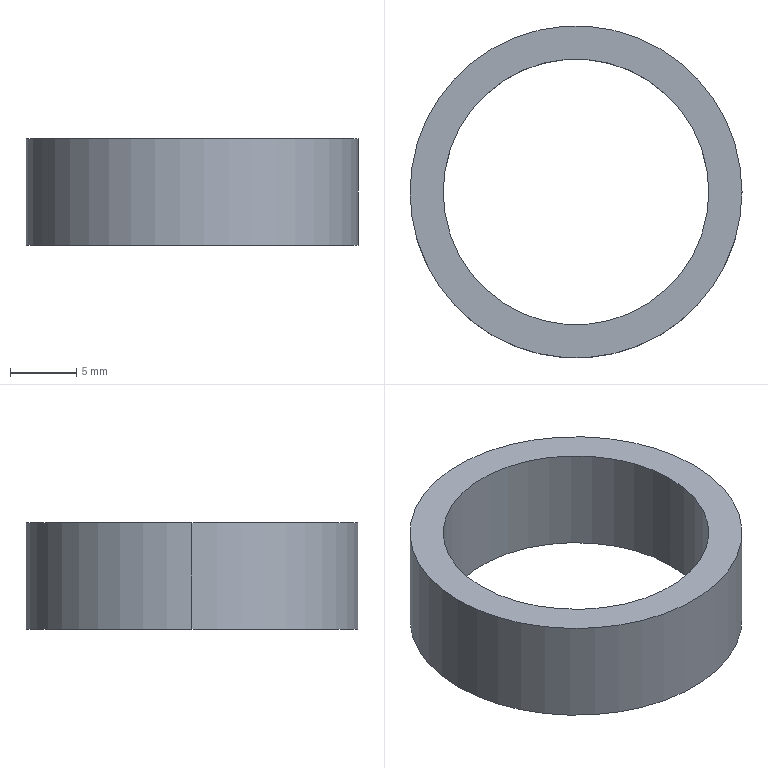Part | STEP file | BCC3 H16_5 | 1 solid | 6 faces | box 25 x 25 x 8 mm | volume 1414 mm3 | cylinder 4 | plane 2 | commonest cylinder face diameters 20 x2 25 x2
STEP:
#1=CARTESIAN_POINT('',(0.,0.,0.));
#2=DIRECTION('',(0.,0.,1.));
#3=DIRECTION('',(1.,0.,0.));
#4=AXIS2_PLACEMENT_3D('',#1,#2,#3);
#5=CARTESIAN_POINT('',(-10.,0.,8.));
#6=VERTEX_POINT('',#5);
#7=CARTESIAN_POINT('',(-10.,0.,0.));
#8=VERTEX_POINT('',#7);
#9=CARTESIAN_POINT('',(-10.,0.,8.));
#10=DIRECTION('',(0.,0.,-1.));
#11=VECTOR('',#10,1.);
#12=LINE('',#9,#11);
#13=CARTESIAN_POINT('',(0.,0.,8.));
#14=DIRECTION('',(0.,0.,-1.));
#15=DIRECTION('',(-1.,0.,0.));
#16=AXIS2_PLACEMENT_3D('',#13,#14,#15);
#17=CYLINDRICAL_SURFACE('',#16,10.);
#18=CARTESIAN_POINT('',(6.283,0.));
#19=DIRECTION('',(0.,1.));
#20=VECTOR('',#19,1.);
#21=LINE('',#18,#20);
#22=(GEOMETRIC_REPRESENTATION_CONTEXT(2)PARAMETRIC_REPRESENTATION_CONTEXT()REPRESENTATION_CONTEXT('',''));
#23=DEFINITIONAL_REPRESENTATION('',(#21),#22);
#24=PCURVE('',#17,#23);
#25=CARTESIAN_POINT('',(0.,0.,8.));
#26=DIRECTION('',(0.,0.,-1.));
#27=DIRECTION('',(-1.,0.,0.));
#28=AXIS2_PLACEMENT_3D('',#25,#26,#27);
#29=CYLINDRICAL_SURFACE('',#28,10.);
#30=CARTESIAN_POINT('',(0.,0.));
#31=DIRECTION('',(0.,1.));
#32=VECTOR('',#31,1.);
#33=LINE('',#30,#32);
#34=(GEOMETRIC_REPRESENTATION_CONTEXT(2)PARAMETRIC_REPRESENTATION_CONTEXT()REPRESENTATION_CONTEXT('',''));
#35=DEFINITIONAL_REPRESENTATION('',(#33),#34);
#36=PCURVE('',#29,#35);
#37=SURFACE_CURVE('',#12,(#24,#36),.PCURVE_S1.);
#38=EDGE_CURVE('',#6,#8,#37,.T.);
#39=ORIENTED_EDGE('',*,*,#38,.T.);
#40=CARTESIAN_POINT('',(10.,0.,0.));
#41=VERTEX_POINT('',#40);
#42=CARTESIAN_POINT('',(0.,0.,0.));
#43=DIRECTION('',(0.,0.,1.));
#44=DIRECTION('',(1.,0.,0.));
#45=AXIS2_PLACEMENT_3D('',#42,#43,#44);
#46=CIRCLE('',#45,10.);
#47=CARTESIAN_POINT('',(9.425,8.));
#48=DIRECTION('',(-1.,0.));
#49=VECTOR('',#48,1.);
#50=LINE('',#47,#49);
#51=(GEOMETRIC_REPRESENTATION_CONTEXT(2)PARAMETRIC_REPRESENTATION_CONTEXT()REPRESENTATION_CONTEXT('',''));
#52=DEFINITIONAL_REPRESENTATION('',(#50),#51);
#53=PCURVE('',#17,#52);
#54=CARTESIAN_POINT('',(0.,0.,0.));
#55=DIRECTION('',(0.,0.,1.));
#56=DIRECTION('',(1.,0.,0.));
#57=AXIS2_PLACEMENT_3D('',#54,#55,#56);
#58=PLANE('',#57);
#59=CARTESIAN_POINT('',(0.,0.));
#60=DIRECTION('',(1.,0.));
#61=AXIS2_PLACEMENT_2D('',#59,#60);
#62=CIRCLE('',#61,10.);
#63=(GEOMETRIC_REPRESENTATION_CONTEXT(2)PARAMETRIC_REPRESENTATION_CONTEXT()REPRESENTATION_CONTEXT('',''));
#64=DEFINITIONAL_REPRESENTATION('',(#62),#63);
#65=PCURVE('',#58,#64);
#66=SURFACE_CURVE('',#46,(#53,#65),.PCURVE_S1.);
#67=EDGE_CURVE('',#8,#41,#66,.T.);
#68=ORIENTED_EDGE('',*,*,#67,.T.);
#69=CARTESIAN_POINT('',(10.,0.,8.));
#70=VERTEX_POINT('',#69);
#71=CARTESIAN_POINT('',(10.,0.,8.));
#72=DIRECTION('',(0.,0.,-1.));
#73=VECTOR('',#72,1.);
#74=LINE('',#71,#73);
#75=CARTESIAN_POINT('',(3.142,0.));
#76=DIRECTION('',(0.,1.));
#77=VECTOR('',#76,1.);
#78=LINE('',#75,#77);
#79=(GEOMETRIC_REPRESENTATION_CONTEXT(2)PARAMETRIC_REPRESENTATION_CONTEXT()REPRESENTATION_CONTEXT('',''));
#80=DEFINITIONAL_REPRESENTATION('',(#78),#79);
#81=PCURVE('',#17,#80);
#82=CARTESIAN_POINT('',(3.142,0.));
#83=DIRECTION('',(0.,1.));
#84=VECTOR('',#83,1.);
#85=LINE('',#82,#84);
#86=(GEOMETRIC_REPRESENTATION_CONTEXT(2)PARAMETRIC_REPRESENTATION_CONTEXT()REPRESENTATION_CONTEXT('',''));
#87=DEFINITIONAL_REPRESENTATION('',(#85),#86);
#88=PCURVE('',#29,#87);
#89=SURFACE_CURVE('',#74,(#81,#88),.PCURVE_S1.);
#90=EDGE_CURVE('',#70,#41,#89,.T.);
#91=ORIENTED_EDGE('',*,*,#90,.F.);
#92=CARTESIAN_POINT('',(0.,0.,8.));
#93=DIRECTION('',(0.,0.,1.));
#94=DIRECTION('',(1.,0.,0.));
#95=AXIS2_PLACEMENT_3D('',#92,#93,#94);
#96=CIRCLE('',#95,10.);
#97=CARTESIAN_POINT('',(9.425,0.));
#98=DIRECTION('',(-1.,0.));
#99=VECTOR('',#98,1.);
#100=LINE('',#97,#99);
#101=(GEOMETRIC_REPRESENTATION_CONTEXT(2)PARAMETRIC_REPRESENTATION_CONTEXT()REPRESENTATION_CONTEXT('',''));
#102=DEFINITIONAL_REPRESENTATION('',(#100),#101);
#103=PCURVE('',#17,#102);
#104=CARTESIAN_POINT('',(0.,0.,8.));
#105=DIRECTION('',(0.,0.,1.));
#106=DIRECTION('',(1.,0.,0.));
#107=AXIS2_PLACEMENT_3D('',#104,#105,#106);
#108=PLANE('',#107);
#109=CARTESIAN_POINT('',(0.,0.));
#110=DIRECTION('',(1.,0.));
#111=AXIS2_PLACEMENT_2D('',#109,#110);
#112=CIRCLE('',#111,10.);
#113=(GEOMETRIC_REPRESENTATION_CONTEXT(2)PARAMETRIC_REPRESENTATION_CONTEXT()REPRESENTATION_CONTEXT('',''));
#114=DEFINITIONAL_REPRESENTATION('',(#112),#113);
#115=PCURVE('',#108,#114);
#116=SURFACE_CURVE('',#96,(#103,#115),.PCURVE_S1.);
#117=EDGE_CURVE('',#6,#70,#116,.T.);
#118=ORIENTED_EDGE('',*,*,#117,.F.);
#119=EDGE_LOOP('',(#39,#68,#91,#118));
#120=FACE_BOUND('',#119,.F.);
#121=ADVANCED_FACE('',(#120),#17,.F.);
#122=CARTESIAN_POINT('',(12.5,0.,8.));
#123=VERTEX_POINT('',#122);
#124=CARTESIAN_POINT('',(-12.5,0.,8.));
#125=VERTEX_POINT('',#124);
#126=CARTESIAN_POINT('',(0.,0.,8.));
#127=DIRECTION('',(0.,0.,1.));
#128=DIRECTION('',(1.,0.,0.));
#129=AXIS2_PLACEMENT_3D('',#126,#127,#128);
#130=CIRCLE('',#129,12.5);
#131=CARTESIAN_POINT('',(0.,0.,8.));
#132=DIRECTION('',(0.,0.,-1.));
#133=DIRECTION('',(-1.,0.,0.));
#134=AXIS2_PLACEMENT_3D('',#131,#132,#133);
#135=CYLINDRICAL_SURFACE('',#134,12.5);
#136=CARTESIAN_POINT('',(3.142,0.));
#137=DIRECTION('',(-1.,0.));
#138=VECTOR('',#137,1.);
#139=LINE('',#136,#138);
#140=(GEOMETRIC_REPRESENTATION_CONTEXT(2)PARAMETRIC_REPRESENTATION_CONTEXT()REPRESENTATION_CONTEXT('',''));
#141=DEFINITIONAL_REPRESENTATION('',(#139),#140);
#142=PCURVE('',#135,#141);
#143=CARTESIAN_POINT('',(0.,0.));
#144=DIRECTION('',(1.,0.));
#145=AXIS2_PLACEMENT_2D('',#143,#144);
#146=CIRCLE('',#145,12.5);
#147=(GEOMETRIC_REPRESENTATION_CONTEXT(2)PARAMETRIC_REPRESENTATION_CONTEXT()REPRESENTATION_CONTEXT('',''));
#148=DEFINITIONAL_REPRESENTATION('',(#146),#147);
#149=PCURVE('',#108,#148);
#150=SURFACE_CURVE('',#130,(#142,#149),.PCURVE_S1.);
#151=EDGE_CURVE('',#123,#125,#150,.T.);
#152=ORIENTED_EDGE('',*,*,#151,.F.);
#153=CARTESIAN_POINT('',(12.5,0.,0.));
#154=VERTEX_POINT('',#153);
#155=CARTESIAN_POINT('',(12.5,0.,8.));
#156=DIRECTION('',(0.,0.,-1.));
#157=VECTOR('',#156,1.);
#158=LINE('',#155,#157);
#159=CARTESIAN_POINT('',(3.142,0.));
#160=DIRECTION('',(0.,1.));
#161=VECTOR('',#160,1.);
#162=LINE('',#159,#161);
#163=(GEOMETRIC_REPRESENTATION_CONTEXT(2)PARAMETRIC_REPRESENTATION_CONTEXT()REPRESENTATION_CONTEXT('',''));
#164=DEFINITIONAL_REPRESENTATION('',(#162),#163);
#165=PCURVE('',#135,#164);
#166=CARTESIAN_POINT('',(0.,0.,8.));
#167=DIRECTION('',(0.,0.,-1.));
#168=DIRECTION('',(-1.,0.,0.));
#169=AXIS2_PLACEMENT_3D('',#166,#167,#168);
#170=CYLINDRICAL_SURFACE('',#169,12.5);
#171=CARTESIAN_POINT('',(3.142,0.));
#172=DIRECTION('',(0.,1.));
#173=VECTOR('',#172,1.);
#174=LINE('',#171,#173);
#175=(GEOMETRIC_REPRESENTATION_CONTEXT(2)PARAMETRIC_REPRESENTATION_CONTEXT()REPRESENTATION_CONTEXT('',''));
#176=DEFINITIONAL_REPRESENTATION('',(#174),#175);
#177=PCURVE('',#170,#176);
#178=SURFACE_CURVE('',#158,(#165,#177),.PCURVE_S1.);
#179=EDGE_CURVE('',#123,#154,#178,.T.);
#180=ORIENTED_EDGE('',*,*,#179,.T.);
#181=CARTESIAN_POINT('',(-12.5,0.,0.));
#182=VERTEX_POINT('',#181);
#183=CARTESIAN_POINT('',(0.,0.,0.));
#184=DIRECTION('',(0.,0.,1.));
#185=DIRECTION('',(1.,0.,0.));
#186=AXIS2_PLACEMENT_3D('',#183,#184,#185);
#187=CIRCLE('',#186,12.5);
#188=CARTESIAN_POINT('',(3.142,8.));
#189=DIRECTION('',(-1.,0.));
#190=VECTOR('',#189,1.);
#191=LINE('',#188,#190);
#192=(GEOMETRIC_REPRESENTATION_CONTEXT(2)PARAMETRIC_REPRESENTATION_CONTEXT()REPRESENTATION_CONTEXT('',''));
#193=DEFINITIONAL_REPRESENTATION('',(#191),#192);
#194=PCURVE('',#135,#193);
#195=CARTESIAN_POINT('',(0.,0.));
#196=DIRECTION('',(1.,0.));
#197=AXIS2_PLACEMENT_2D('',#195,#196);
#198=CIRCLE('',#197,12.5);
#199=(GEOMETRIC_REPRESENTATION_CONTEXT(2)PARAMETRIC_REPRESENTATION_CONTEXT()REPRESENTATION_CONTEXT('',''));
#200=DEFINITIONAL_REPRESENTATION('',(#198),#199);
#201=PCURVE('',#58,#200);
#202=SURFACE_CURVE('',#187,(#194,#201),.PCURVE_S1.);
#203=EDGE_CURVE('',#154,#182,#202,.T.);
#204=ORIENTED_EDGE('',*,*,#203,.T.);
#205=CARTESIAN_POINT('',(-12.5,0.,8.));
#206=DIRECTION('',(0.,0.,-1.));
#207=VECTOR('',#206,1.);
#208=LINE('',#205,#207);
#209=CARTESIAN_POINT('',(0.,0.));
#210=DIRECTION('',(0.,1.));
#211=VECTOR('',#210,1.);
#212=LINE('',#209,#211);
#213=(GEOMETRIC_REPRESENTATION_CONTEXT(2)PARAMETRIC_REPRESENTATION_CONTEXT()REPRESENTATION_CONTEXT('',''));
#214=DEFINITIONAL_REPRESENTATION('',(#212),#213);
#215=PCURVE('',#135,#214);
#216=CARTESIAN_POINT('',(6.283,0.));
#217=DIRECTION('',(0.,1.));
#218=VECTOR('',#217,1.);
#219=LINE('',#216,#218);
#220=(GEOMETRIC_REPRESENTATION_CONTEXT(2)PARAMETRIC_REPRESENTATION_CONTEXT()REPRESENTATION_CONTEXT('',''));
#221=DEFINITIONAL_REPRESENTATION('',(#219),#220);
#222=PCURVE('',#170,#221);
#223=SURFACE_CURVE('',#208,(#215,#222),.PCURVE_S1.);
#224=EDGE_CURVE('',#125,#182,#223,.T.);
#225=ORIENTED_EDGE('',*,*,#224,.F.);
#226=EDGE_LOOP('',(#152,#180,#204,#225));
#227=FACE_BOUND('',#226,.T.);
#228=ADVANCED_FACE('',(#227),#135,.T.);
#229=CARTESIAN_POINT('',(0.,0.,8.));
#230=DIRECTION('',(0.,0.,1.));
#231=DIRECTION('',(1.,0.,0.));
#232=AXIS2_PLACEMENT_3D('',#229,#230,#231);
#233=CIRCLE('',#232,12.5);
#234=CARTESIAN_POINT('',(0.,0.));
#235=DIRECTION('',(1.,0.));
#236=AXIS2_PLACEMENT_2D('',#234,#235);
#237=CIRCLE('',#236,12.5);
#238=(GEOMETRIC_REPRESENTATION_CONTEXT(2)PARAMETRIC_REPRESENTATION_CONTEXT()REPRESENTATION_CONTEXT('',''));
#239=DEFINITIONAL_REPRESENTATION('',(#237),#238);
#240=PCURVE('',#108,#239);
#241=CARTESIAN_POINT('',(9.425,0.));
#242=DIRECTION('',(-1.,0.));
#243=VECTOR('',#242,1.);
#244=LINE('',#241,#243);
#245=(GEOMETRIC_REPRESENTATION_CONTEXT(2)PARAMETRIC_REPRESENTATION_CONTEXT()REPRESENTATION_CONTEXT('',''));
#246=DEFINITIONAL_REPRESENTATION('',(#244),#245);
#247=PCURVE('',#170,#246);
#248=SURFACE_CURVE('',#233,(#240,#247),.PCURVE_S1.);
#249=EDGE_CURVE('',#125,#123,#248,.T.);
#250=ORIENTED_EDGE('',*,*,#249,.T.);
#251=ORIENTED_EDGE('',*,*,#151,.T.);
#252=EDGE_LOOP('',(#250,#251));
#253=FACE_BOUND('',#252,.T.);
#254=ORIENTED_EDGE('',*,*,#117,.F.);
#255=CARTESIAN_POINT('',(0.,0.,8.));
#256=DIRECTION('',(0.,0.,1.));
#257=DIRECTION('',(1.,0.,0.));
#258=AXIS2_PLACEMENT_3D('',#255,#256,#257);
#259=CIRCLE('',#258,10.);
#260=CARTESIAN_POINT('',(0.,0.));
#261=DIRECTION('',(1.,0.));
#262=AXIS2_PLACEMENT_2D('',#260,#261);
#263=CIRCLE('',#262,10.);
#264=(GEOMETRIC_REPRESENTATION_CONTEXT(2)PARAMETRIC_REPRESENTATION_CONTEXT()REPRESENTATION_CONTEXT('',''));
#265=DEFINITIONAL_REPRESENTATION('',(#263),#264);
#266=PCURVE('',#108,#265);
#267=CARTESIAN_POINT('',(3.142,0.));
#268=DIRECTION('',(-1.,0.));
#269=VECTOR('',#268,1.);
#270=LINE('',#267,#269);
#271=(GEOMETRIC_REPRESENTATION_CONTEXT(2)PARAMETRIC_REPRESENTATION_CONTEXT()REPRESENTATION_CONTEXT('',''));
#272=DEFINITIONAL_REPRESENTATION('',(#270),#271);
#273=PCURVE('',#29,#272);
#274=SURFACE_CURVE('',#259,(#266,#273),.PCURVE_S1.);
#275=EDGE_CURVE('',#70,#6,#274,.T.);
#276=ORIENTED_EDGE('',*,*,#275,.F.);
#277=EDGE_LOOP('',(#254,#276));
#278=FACE_BOUND('',#277,.T.);
#279=ADVANCED_FACE('',(#253,#278),#108,.T.);
#280=CARTESIAN_POINT('',(0.,0.,0.));
#281=DIRECTION('',(0.,0.,1.));
#282=DIRECTION('',(1.,0.,0.));
#283=AXIS2_PLACEMENT_3D('',#280,#281,#282);
#284=CIRCLE('',#283,12.5);
#285=CARTESIAN_POINT('',(0.,0.));
#286=DIRECTION('',(1.,0.));
#287=AXIS2_PLACEMENT_2D('',#285,#286);
#288=CIRCLE('',#287,12.5);
#289=(GEOMETRIC_REPRESENTATION_CONTEXT(2)PARAMETRIC_REPRESENTATION_CONTEXT()REPRESENTATION_CONTEXT('',''));
#290=DEFINITIONAL_REPRESENTATION('',(#288),#289);
#291=PCURVE('',#58,#290);
#292=CARTESIAN_POINT('',(9.425,8.));
#293=DIRECTION('',(-1.,0.));
#294=VECTOR('',#293,1.);
#295=LINE('',#292,#294);
#296=(GEOMETRIC_REPRESENTATION_CONTEXT(2)PARAMETRIC_REPRESENTATION_CONTEXT()REPRESENTATION_CONTEXT('',''));
#297=DEFINITIONAL_REPRESENTATION('',(#295),#296);
#298=PCURVE('',#170,#297);
#299=SURFACE_CURVE('',#284,(#291,#298),.PCURVE_S1.);
#300=EDGE_CURVE('',#182,#154,#299,.T.);
#301=ORIENTED_EDGE('',*,*,#300,.F.);
#302=ORIENTED_EDGE('',*,*,#203,.F.);
#303=EDGE_LOOP('',(#301,#302));
#304=FACE_BOUND('',#303,.T.);
#305=ORIENTED_EDGE('',*,*,#67,.T.);
#306=CARTESIAN_POINT('',(0.,0.,0.));
#307=DIRECTION('',(0.,0.,1.));
#308=DIRECTION('',(1.,0.,0.));
#309=AXIS2_PLACEMENT_3D('',#306,#307,#308);
#310=CIRCLE('',#309,10.);
#311=CARTESIAN_POINT('',(0.,0.));
#312=DIRECTION('',(1.,0.));
#313=AXIS2_PLACEMENT_2D('',#311,#312);
#314=CIRCLE('',#313,10.);
#315=(GEOMETRIC_REPRESENTATION_CONTEXT(2)PARAMETRIC_REPRESENTATION_CONTEXT()REPRESENTATION_CONTEXT('',''));
#316=DEFINITIONAL_REPRESENTATION('',(#314),#315);
#317=PCURVE('',#58,#316);
#318=CARTESIAN_POINT('',(3.142,8.));
#319=DIRECTION('',(-1.,0.));
#320=VECTOR('',#319,1.);
#321=LINE('',#318,#320);
#322=(GEOMETRIC_REPRESENTATION_CONTEXT(2)PARAMETRIC_REPRESENTATION_CONTEXT()REPRESENTATION_CONTEXT('',''));
#323=DEFINITIONAL_REPRESENTATION('',(#321),#322);
#324=PCURVE('',#29,#323);
#325=SURFACE_CURVE('',#310,(#317,#324),.PCURVE_S1.);
#326=EDGE_CURVE('',#41,#8,#325,.T.);
#327=ORIENTED_EDGE('',*,*,#326,.T.);
#328=EDGE_LOOP('',(#305,#327));
#329=FACE_BOUND('',#328,.T.);
#330=ADVANCED_FACE('',(#304,#329),#58,.F.);
#331=ORIENTED_EDGE('',*,*,#179,.F.);
#332=ORIENTED_EDGE('',*,*,#249,.F.);
#333=ORIENTED_EDGE('',*,*,#224,.T.);
#334=ORIENTED_EDGE('',*,*,#300,.T.);
#335=EDGE_LOOP('',(#331,#332,#333,#334));
#336=FACE_BOUND('',#335,.T.);
#337=ADVANCED_FACE('',(#336),#170,.T.);
#338=ORIENTED_EDGE('',*,*,#326,.T.);
#339=ORIENTED_EDGE('',*,*,#38,.F.);
#340=ORIENTED_EDGE('',*,*,#275,.F.);
#341=ORIENTED_EDGE('',*,*,#90,.T.);
#342=EDGE_LOOP('',(#338,#339,#340,#341));
#343=FACE_BOUND('',#342,.F.);
#344=ADVANCED_FACE('',(#343),#29,.F.);
#345=CLOSED_SHELL('',(#121,#228,#279,#330,#337,#344));
#346=MANIFOLD_SOLID_BREP('',#345);
#347=(LENGTH_UNIT()NAMED_UNIT(*)SI_UNIT(.MILLI.,.METRE.));
#348=UNCERTAINTY_MEASURE_WITH_UNIT(LENGTH_MEASURE(0.0000001),#347,'','');
#349=(NAMED_UNIT(*)PLANE_ANGLE_UNIT()SI_UNIT($,.RADIAN.));
#350=(NAMED_UNIT(*)SI_UNIT($,.STERADIAN.)SOLID_ANGLE_UNIT());
#351=(GEOMETRIC_REPRESENTATION_CONTEXT(3)GLOBAL_UNCERTAINTY_ASSIGNED_CONTEXT((#348))GLOBAL_UNIT_ASSIGNED_CONTEXT((#347,#349,#350))REPRESENTATION_CONTEXT('',''));
#352=ADVANCED_BREP_SHAPE_REPRESENTATION('',(#4,#346),#351);